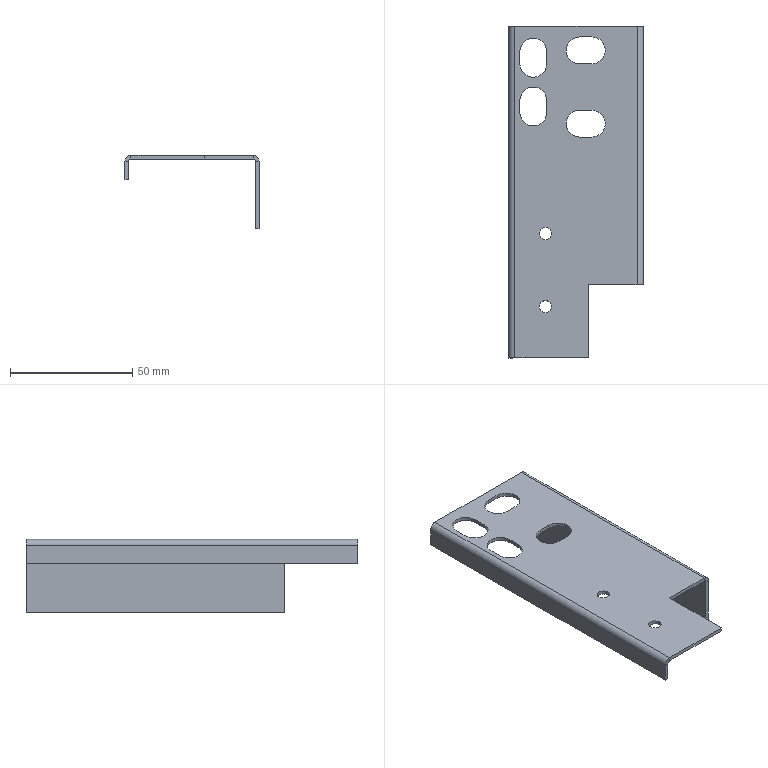Part | SolidWorks | features Cut 4, EdgeFlange 2, FlatPattern 1, SMBaseFlange 1, SheetMetal 1 | 1 solid | 46 faces | box 55 x 136 x 30 mm | volume 15241 mm3 | plane 28 | cylinder 18 | commonest cylinder face diameters 11 x10 5 x6 2 x2
STEP:
#1=CARTESIAN_POINT('',(12.,58.,-1.5));
#2=VERTEX_POINT('',#1);
#3=CARTESIAN_POINT('',(6.5,63.5,-1.5));
#4=VERTEX_POINT('',#3);
#5=CARTESIAN_POINT('',(6.5,58.,-1.5));
#6=DIRECTION('',(0.,0.,1.));
#7=DIRECTION('',(1.,0.,0.));
#8=AXIS2_PLACEMENT_3D('',#5,#6,#7);
#9=CIRCLE('',#8,5.5);
#10=EDGE_CURVE('',#2,#4,#9,.T.);
#11=ORIENTED_EDGE('',*,*,#10,.F.);
#12=CARTESIAN_POINT('',(12.,58.,0.));
#13=VERTEX_POINT('',#12);
#14=CARTESIAN_POINT('',(12.,58.,-10.));
#15=DIRECTION('',(0.,0.,1.));
#16=VECTOR('',#15,1000.);
#17=LINE('',#14,#16);
#18=EDGE_CURVE('',#2,#13,#17,.T.);
#19=ORIENTED_EDGE('',*,*,#18,.T.);
#20=CARTESIAN_POINT('',(6.5,63.5,0.));
#21=VERTEX_POINT('',#20);
#22=CARTESIAN_POINT('',(6.5,58.,0.));
#23=DIRECTION('',(0.,0.,1.));
#24=DIRECTION('',(1.,0.,0.));
#25=AXIS2_PLACEMENT_3D('',#22,#23,#24);
#26=CIRCLE('',#25,5.5);
#27=EDGE_CURVE('',#13,#21,#26,.T.);
#28=ORIENTED_EDGE('',*,*,#27,.T.);
#29=CARTESIAN_POINT('',(6.5,63.5,-10.));
#30=DIRECTION('',(0.,0.,1.));
#31=VECTOR('',#30,1000.);
#32=LINE('',#29,#31);
#33=EDGE_CURVE('',#4,#21,#32,.T.);
#34=ORIENTED_EDGE('',*,*,#33,.F.);
#35=EDGE_LOOP('',(#11,#19,#28,#34));
#36=FACE_OUTER_BOUND('',#35,.T.);
#37=CARTESIAN_POINT('',(6.5,58.,-10.));
#38=DIRECTION('',(0.,0.,1.));
#39=DIRECTION('',(1.,0.,0.));
#40=AXIS2_PLACEMENT_3D('',#37,#38,#39);
#41=CYLINDRICAL_SURFACE('',#40,5.5);
#42=ADVANCED_FACE('',(#36),#41,.F.);
#43=CARTESIAN_POINT('',(12.,28.,-1.5));
#44=VERTEX_POINT('',#43);
#45=CARTESIAN_POINT('',(6.5,33.5,-1.5));
#46=VERTEX_POINT('',#45);
#47=CARTESIAN_POINT('',(6.5,28.,-1.5));
#48=DIRECTION('',(0.,0.,1.));
#49=DIRECTION('',(1.,0.,0.));
#50=AXIS2_PLACEMENT_3D('',#47,#48,#49);
#51=CIRCLE('',#50,5.5);
#52=EDGE_CURVE('',#44,#46,#51,.T.);
#53=ORIENTED_EDGE('',*,*,#52,.F.);
#54=CARTESIAN_POINT('',(12.,28.,0.));
#55=VERTEX_POINT('',#54);
#56=CARTESIAN_POINT('',(12.,28.,-10.));
#57=DIRECTION('',(0.,0.,1.));
#58=VECTOR('',#57,1000.);
#59=LINE('',#56,#58);
#60=EDGE_CURVE('',#44,#55,#59,.T.);
#61=ORIENTED_EDGE('',*,*,#60,.T.);
#62=CARTESIAN_POINT('',(6.5,33.5,0.));
#63=VERTEX_POINT('',#62);
#64=CARTESIAN_POINT('',(6.5,28.,0.));
#65=DIRECTION('',(0.,0.,1.));
#66=DIRECTION('',(1.,0.,0.));
#67=AXIS2_PLACEMENT_3D('',#64,#65,#66);
#68=CIRCLE('',#67,5.5);
#69=EDGE_CURVE('',#55,#63,#68,.T.);
#70=ORIENTED_EDGE('',*,*,#69,.T.);
#71=CARTESIAN_POINT('',(6.5,33.5,-10.));
#72=DIRECTION('',(0.,0.,1.));
#73=VECTOR('',#72,1000.);
#74=LINE('',#71,#73);
#75=EDGE_CURVE('',#46,#63,#74,.T.);
#76=ORIENTED_EDGE('',*,*,#75,.F.);
#77=EDGE_LOOP('',(#53,#61,#70,#76));
#78=FACE_OUTER_BOUND('',#77,.T.);
#79=CARTESIAN_POINT('',(6.5,28.,-10.));
#80=DIRECTION('',(0.,0.,1.));
#81=DIRECTION('',(1.,0.,0.));
#82=AXIS2_PLACEMENT_3D('',#79,#80,#81);
#83=CYLINDRICAL_SURFACE('',#82,5.5);
#84=ADVANCED_FACE('',(#78),#83,.F.);
#85=CARTESIAN_POINT('',(-15.,-47.,-1.5));
#86=VERTEX_POINT('',#85);
#87=CARTESIAN_POINT('',(-10.,-47.,-1.5));
#88=VERTEX_POINT('',#87);
#89=CARTESIAN_POINT('',(-12.5,-47.,-1.5));
#90=DIRECTION('',(0.,0.,1.));
#91=DIRECTION('',(1.,0.,0.));
#92=AXIS2_PLACEMENT_3D('',#89,#90,#91);
#93=CIRCLE('',#92,2.5);
#94=EDGE_CURVE('',#86,#88,#93,.T.);
#95=ORIENTED_EDGE('',*,*,#94,.F.);
#96=CARTESIAN_POINT('',(-15.,-47.,0.));
#97=VERTEX_POINT('',#96);
#98=CARTESIAN_POINT('',(-15.,-47.,-10.));
#99=DIRECTION('',(0.,0.,1.));
#100=VECTOR('',#99,1000.);
#101=LINE('',#98,#100);
#102=EDGE_CURVE('',#86,#97,#101,.T.);
#103=ORIENTED_EDGE('',*,*,#102,.T.);
#104=CARTESIAN_POINT('',(-10.,-47.,0.));
#105=VERTEX_POINT('',#104);
#106=CARTESIAN_POINT('',(-12.5,-47.,0.));
#107=DIRECTION('',(0.,0.,1.));
#108=DIRECTION('',(1.,0.,0.));
#109=AXIS2_PLACEMENT_3D('',#106,#107,#108);
#110=CIRCLE('',#109,2.5);
#111=EDGE_CURVE('',#97,#105,#110,.T.);
#112=ORIENTED_EDGE('',*,*,#111,.T.);
#113=CARTESIAN_POINT('',(-10.,-47.,-10.));
#114=DIRECTION('',(0.,0.,1.));
#115=VECTOR('',#114,1000.);
#116=LINE('',#113,#115);
#117=EDGE_CURVE('',#88,#105,#116,.T.);
#118=ORIENTED_EDGE('',*,*,#117,.F.);
#119=EDGE_LOOP('',(#95,#103,#112,#118));
#120=FACE_OUTER_BOUND('',#119,.T.);
#121=CARTESIAN_POINT('',(-12.5,-47.,-10.));
#122=DIRECTION('',(0.,0.,1.));
#123=DIRECTION('',(1.,0.,0.));
#124=AXIS2_PLACEMENT_3D('',#121,#122,#123);
#125=CYLINDRICAL_SURFACE('',#124,2.5);
#126=ADVANCED_FACE('',(#120),#125,.F.);
#127=CARTESIAN_POINT('',(-15.,-17.,-1.5));
#128=VERTEX_POINT('',#127);
#129=CARTESIAN_POINT('',(-10.,-17.,-1.5));
#130=VERTEX_POINT('',#129);
#131=CARTESIAN_POINT('',(-12.5,-17.,-1.5));
#132=DIRECTION('',(0.,0.,1.));
#133=DIRECTION('',(1.,0.,0.));
#134=AXIS2_PLACEMENT_3D('',#131,#132,#133);
#135=CIRCLE('',#134,2.5);
#136=EDGE_CURVE('',#128,#130,#135,.T.);
#137=ORIENTED_EDGE('',*,*,#136,.F.);
#138=CARTESIAN_POINT('',(-15.,-17.,0.));
#139=VERTEX_POINT('',#138);
#140=CARTESIAN_POINT('',(-15.,-17.,-10.));
#141=DIRECTION('',(0.,0.,1.));
#142=VECTOR('',#141,1000.);
#143=LINE('',#140,#142);
#144=EDGE_CURVE('',#128,#139,#143,.T.);
#145=ORIENTED_EDGE('',*,*,#144,.T.);
#146=CARTESIAN_POINT('',(-10.,-17.,0.));
#147=VERTEX_POINT('',#146);
#148=CARTESIAN_POINT('',(-12.5,-17.,0.));
#149=DIRECTION('',(0.,0.,1.));
#150=DIRECTION('',(1.,0.,0.));
#151=AXIS2_PLACEMENT_3D('',#148,#149,#150);
#152=CIRCLE('',#151,2.5);
#153=EDGE_CURVE('',#139,#147,#152,.T.);
#154=ORIENTED_EDGE('',*,*,#153,.T.);
#155=CARTESIAN_POINT('',(-10.,-17.,-10.));
#156=DIRECTION('',(0.,0.,1.));
#157=VECTOR('',#156,1000.);
#158=LINE('',#155,#157);
#159=EDGE_CURVE('',#130,#147,#158,.T.);
#160=ORIENTED_EDGE('',*,*,#159,.F.);
#161=EDGE_LOOP('',(#137,#145,#154,#160));
#162=FACE_OUTER_BOUND('',#161,.T.);
#163=CARTESIAN_POINT('',(-12.5,-17.,-10.));
#164=DIRECTION('',(0.,0.,1.));
#165=DIRECTION('',(1.,0.,0.));
#166=AXIS2_PLACEMENT_3D('',#163,#164,#165);
#167=CYLINDRICAL_SURFACE('',#166,2.5);
#168=ADVANCED_FACE('',(#162),#167,.F.);
#169=CARTESIAN_POINT('',(27.5,-38.,-30.));
#170=VERTEX_POINT('',#169);
#171=CARTESIAN_POINT('',(27.5,-38.,-2.5));
#172=VERTEX_POINT('',#171);
#173=CARTESIAN_POINT('',(27.5,-38.,-30.));
#174=DIRECTION('',(0.,0.,1.));
#175=VECTOR('',#174,1000.);
#176=LINE('',#173,#175);
#177=EDGE_CURVE('',#170,#172,#176,.T.);
#178=ORIENTED_EDGE('',*,*,#177,.T.);
#179=CARTESIAN_POINT('',(26.,-38.,-2.5));
#180=VERTEX_POINT('',#179);
#181=CARTESIAN_POINT('',(27.5,-38.,-2.5));
#182=DIRECTION('',(-1.,0.,0.));
#183=VECTOR('',#182,1000.);
#184=LINE('',#181,#183);
#185=EDGE_CURVE('',#172,#180,#184,.T.);
#186=ORIENTED_EDGE('',*,*,#185,.T.);
#187=CARTESIAN_POINT('',(26.,-38.,-30.));
#188=VERTEX_POINT('',#187);
#189=CARTESIAN_POINT('',(26.,-38.,0.));
#190=DIRECTION('',(0.,0.,1.));
#191=VECTOR('',#190,1000.);
#192=LINE('',#189,#191);
#193=EDGE_CURVE('',#188,#180,#192,.T.);
#194=ORIENTED_EDGE('',*,*,#193,.F.);
#195=CARTESIAN_POINT('',(27.5,-38.,-30.));
#196=DIRECTION('',(-1.,0.,0.));
#197=VECTOR('',#196,1000.);
#198=LINE('',#195,#197);
#199=EDGE_CURVE('',#170,#188,#198,.T.);
#200=ORIENTED_EDGE('',*,*,#199,.F.);
#201=EDGE_LOOP('',(#178,#186,#194,#200));
#202=FACE_OUTER_BOUND('',#201,.T.);
#203=CARTESIAN_POINT('',(27.5,-38.,-30.));
#204=DIRECTION('',(0.,1.,0.));
#205=DIRECTION('',(-1.,0.,0.));
#206=AXIS2_PLACEMENT_3D('',#203,#204,#205);
#207=PLANE('',#206);
#208=ADVANCED_FACE('',(#202),#207,.F.);
#209=CARTESIAN_POINT('',(25.,-38.,-1.5));
#210=VERTEX_POINT('',#209);
#211=CARTESIAN_POINT('',(5.,-38.,-1.5));
#212=VERTEX_POINT('',#211);
#213=CARTESIAN_POINT('',(0.,-38.,-1.5));
#214=DIRECTION('',(-1.,0.,0.));
#215=VECTOR('',#214,1000.);
#216=LINE('',#213,#215);
#217=EDGE_CURVE('',#210,#212,#216,.T.);
#218=ORIENTED_EDGE('',*,*,#217,.F.);
#219=CARTESIAN_POINT('',(25.,-38.,0.));
#220=VERTEX_POINT('',#219);
#221=CARTESIAN_POINT('',(25.,-38.,-1.5));
#222=DIRECTION('',(0.,0.,1.));
#223=VECTOR('',#222,1000.);
#224=LINE('',#221,#223);
#225=EDGE_CURVE('',#210,#220,#224,.T.);
#226=ORIENTED_EDGE('',*,*,#225,.T.);
#227=CARTESIAN_POINT('',(5.,-38.,0.));
#228=VERTEX_POINT('',#227);
#229=CARTESIAN_POINT('',(0.,-38.,0.));
#230=DIRECTION('',(-1.,0.,0.));
#231=VECTOR('',#230,1000.);
#232=LINE('',#229,#231);
#233=EDGE_CURVE('',#220,#228,#232,.T.);
#234=ORIENTED_EDGE('',*,*,#233,.T.);
#235=CARTESIAN_POINT('',(5.,-38.,-30.));
#236=DIRECTION('',(0.,0.,1.));
#237=VECTOR('',#236,1000.);
#238=LINE('',#235,#237);
#239=EDGE_CURVE('',#212,#228,#238,.T.);
#240=ORIENTED_EDGE('',*,*,#239,.F.);
#241=EDGE_LOOP('',(#218,#226,#234,#240));
#242=FACE_OUTER_BOUND('',#241,.T.);
#243=CARTESIAN_POINT('',(27.5,-38.,-30.));
#244=DIRECTION('',(0.,1.,0.));
#245=DIRECTION('',(-1.,0.,0.));
#246=AXIS2_PLACEMENT_3D('',#243,#244,#245);
#247=PLANE('',#246);
#248=ADVANCED_FACE('',(#242),#247,.F.);
#249=CARTESIAN_POINT('',(-12.,52.5,-1.5));
#250=VERTEX_POINT('',#249);
#251=CARTESIAN_POINT('',(-12.,57.5,-1.5));
#252=VERTEX_POINT('',#251);
#253=CARTESIAN_POINT('',(-12.,0.,-1.5));
#254=DIRECTION('',(0.,1.,0.));
#255=VECTOR('',#254,1000.);
#256=LINE('',#253,#255);
#257=EDGE_CURVE('',#250,#252,#256,.T.);
#258=ORIENTED_EDGE('',*,*,#257,.T.);
#259=CARTESIAN_POINT('',(-23.,57.5,-1.5));
#260=VERTEX_POINT('',#259);
#261=CARTESIAN_POINT('',(-17.5,57.5,-1.5));
#262=DIRECTION('',(0.,0.,1.));
#263=DIRECTION('',(1.,0.,0.));
#264=AXIS2_PLACEMENT_3D('',#261,#262,#263);
#265=CIRCLE('',#264,5.5);
#266=EDGE_CURVE('',#252,#260,#265,.T.);
#267=ORIENTED_EDGE('',*,*,#266,.T.);
#268=CARTESIAN_POINT('',(-23.,52.5,-1.5));
#269=VERTEX_POINT('',#268);
#270=CARTESIAN_POINT('',(-23.,0.,-1.5));
#271=DIRECTION('',(0.,-1.,0.));
#272=VECTOR('',#271,1000.);
#273=LINE('',#270,#272);
#274=EDGE_CURVE('',#260,#269,#273,.T.);
#275=ORIENTED_EDGE('',*,*,#274,.T.);
#276=CARTESIAN_POINT('',(-17.5,52.5,-1.5));
#277=DIRECTION('',(0.,0.,1.));
#278=DIRECTION('',(1.,0.,0.));
#279=AXIS2_PLACEMENT_3D('',#276,#277,#278);
#280=CIRCLE('',#279,5.5);
#281=EDGE_CURVE('',#269,#250,#280,.T.);
#282=ORIENTED_EDGE('',*,*,#281,.T.);
#283=EDGE_LOOP('',(#258,#267,#275,#282));
#284=FACE_BOUND('',#283,.T.);
#285=CARTESIAN_POINT('',(-12.,32.5,-1.5));
#286=VERTEX_POINT('',#285);
#287=CARTESIAN_POINT('',(-12.,37.5,-1.5));
#288=VERTEX_POINT('',#287);
#289=CARTESIAN_POINT('',(-12.,0.,-1.5));
#290=DIRECTION('',(0.,1.,0.));
#291=VECTOR('',#290,1000.);
#292=LINE('',#289,#291);
#293=EDGE_CURVE('',#286,#288,#292,.T.);
#294=ORIENTED_EDGE('',*,*,#293,.T.);
#295=CARTESIAN_POINT('',(-23.,37.5,-1.5));
#296=VERTEX_POINT('',#295);
#297=CARTESIAN_POINT('',(-17.5,37.5,-1.5));
#298=DIRECTION('',(0.,0.,1.));
#299=DIRECTION('',(1.,0.,0.));
#300=AXIS2_PLACEMENT_3D('',#297,#298,#299);
#301=CIRCLE('',#300,5.5);
#302=EDGE_CURVE('',#288,#296,#301,.T.);
#303=ORIENTED_EDGE('',*,*,#302,.T.);
#304=CARTESIAN_POINT('',(-23.,32.5,-1.5));
#305=VERTEX_POINT('',#304);
#306=CARTESIAN_POINT('',(-23.,0.,-1.5));
#307=DIRECTION('',(0.,-1.,0.));
#308=VECTOR('',#307,1000.);
#309=LINE('',#306,#308);
#310=EDGE_CURVE('',#296,#305,#309,.T.);
#311=ORIENTED_EDGE('',*,*,#310,.T.);
#312=CARTESIAN_POINT('',(-17.5,32.5,-1.5));
#313=DIRECTION('',(0.,0.,1.));
#314=DIRECTION('',(1.,0.,0.));
#315=AXIS2_PLACEMENT_3D('',#312,#313,#314);
#316=CIRCLE('',#315,5.5);
#317=EDGE_CURVE('',#305,#286,#316,.T.);
#318=ORIENTED_EDGE('',*,*,#317,.T.);
#319=EDGE_LOOP('',(#294,#303,#311,#318));
#320=FACE_BOUND('',#319,.T.);
#321=CARTESIAN_POINT('',(1.5,63.5,-1.5));
#322=VERTEX_POINT('',#321);
#323=CARTESIAN_POINT('',(0.,63.5,-1.5));
#324=DIRECTION('',(-1.,0.,0.));
#325=VECTOR('',#324,1000.);
#326=LINE('',#323,#325);
#327=EDGE_CURVE('',#4,#322,#326,.T.);
#328=ORIENTED_EDGE('',*,*,#327,.T.);
#329=CARTESIAN_POINT('',(1.5,52.5,-1.5));
#330=VERTEX_POINT('',#329);
#331=CARTESIAN_POINT('',(1.5,58.,-1.5));
#332=DIRECTION('',(0.,0.,1.));
#333=DIRECTION('',(1.,0.,0.));
#334=AXIS2_PLACEMENT_3D('',#331,#332,#333);
#335=CIRCLE('',#334,5.5);
#336=EDGE_CURVE('',#322,#330,#335,.T.);
#337=ORIENTED_EDGE('',*,*,#336,.T.);
#338=CARTESIAN_POINT('',(6.5,52.5,-1.5));
#339=VERTEX_POINT('',#338);
#340=CARTESIAN_POINT('',(0.,52.5,-1.5));
#341=DIRECTION('',(1.,0.,0.));
#342=VECTOR('',#341,1000.);
#343=LINE('',#340,#342);
#344=EDGE_CURVE('',#330,#339,#343,.T.);
#345=ORIENTED_EDGE('',*,*,#344,.T.);
#346=CARTESIAN_POINT('',(6.5,58.,-1.5));
#347=DIRECTION('',(0.,0.,1.));
#348=DIRECTION('',(1.,0.,0.));
#349=AXIS2_PLACEMENT_3D('',#346,#347,#348);
#350=CIRCLE('',#349,5.5);
#351=EDGE_CURVE('',#339,#2,#350,.T.);
#352=ORIENTED_EDGE('',*,*,#351,.T.);
#353=ORIENTED_EDGE('',*,*,#10,.T.);
#354=EDGE_LOOP('',(#328,#337,#345,#352,#353));
#355=FACE_BOUND('',#354,.T.);
#356=CARTESIAN_POINT('',(1.5,33.5,-1.5));
#357=VERTEX_POINT('',#356);
#358=CARTESIAN_POINT('',(0.,33.5,-1.5));
#359=DIRECTION('',(-1.,0.,0.));
#360=VECTOR('',#359,1000.);
#361=LINE('',#358,#360);
#362=EDGE_CURVE('',#46,#357,#361,.T.);
#363=ORIENTED_EDGE('',*,*,#362,.T.);
#364=CARTESIAN_POINT('',(1.5,22.5,-1.5));
#365=VERTEX_POINT('',#364);
#366=CARTESIAN_POINT('',(1.5,28.,-1.5));
#367=DIRECTION('',(0.,0.,1.));
#368=DIRECTION('',(1.,0.,0.));
#369=AXIS2_PLACEMENT_3D('',#366,#367,#368);
#370=CIRCLE('',#369,5.5);
#371=EDGE_CURVE('',#357,#365,#370,.T.);
#372=ORIENTED_EDGE('',*,*,#371,.T.);
#373=CARTESIAN_POINT('',(6.5,22.5,-1.5));
#374=VERTEX_POINT('',#373);
#375=CARTESIAN_POINT('',(0.,22.5,-1.5));
#376=DIRECTION('',(1.,0.,0.));
#377=VECTOR('',#376,1000.);
#378=LINE('',#375,#377);
#379=EDGE_CURVE('',#365,#374,#378,.T.);
#380=ORIENTED_EDGE('',*,*,#379,.T.);
#381=CARTESIAN_POINT('',(6.5,28.,-1.5));
#382=DIRECTION('',(0.,0.,1.));
#383=DIRECTION('',(1.,0.,0.));
#384=AXIS2_PLACEMENT_3D('',#381,#382,#383);
#385=CIRCLE('',#384,5.5);
#386=EDGE_CURVE('',#374,#44,#385,.T.);
#387=ORIENTED_EDGE('',*,*,#386,.T.);
#388=ORIENTED_EDGE('',*,*,#52,.T.);
#389=EDGE_LOOP('',(#363,#372,#380,#387,#388));
#390=FACE_BOUND('',#389,.T.);
#391=CARTESIAN_POINT('',(-12.5,-47.,-1.5));
#392=DIRECTION('',(0.,0.,1.));
#393=DIRECTION('',(1.,0.,0.));
#394=AXIS2_PLACEMENT_3D('',#391,#392,#393);
#395=CIRCLE('',#394,2.5);
#396=EDGE_CURVE('',#88,#86,#395,.T.);
#397=ORIENTED_EDGE('',*,*,#396,.T.);
#398=ORIENTED_EDGE('',*,*,#94,.T.);
#399=EDGE_LOOP('',(#397,#398));
#400=FACE_BOUND('',#399,.T.);
#401=CARTESIAN_POINT('',(-12.5,-17.,-1.5));
#402=DIRECTION('',(0.,0.,1.));
#403=DIRECTION('',(1.,0.,0.));
#404=AXIS2_PLACEMENT_3D('',#401,#402,#403);
#405=CIRCLE('',#404,2.5);
#406=EDGE_CURVE('',#130,#128,#405,.T.);
#407=ORIENTED_EDGE('',*,*,#406,.T.);
#408=ORIENTED_EDGE('',*,*,#136,.T.);
#409=EDGE_LOOP('',(#407,#408));
#410=FACE_BOUND('',#409,.T.);
#411=ORIENTED_EDGE('',*,*,#217,.T.);
#412=CARTESIAN_POINT('',(5.,-68.,-1.5));
#413=VERTEX_POINT('',#412);
#414=CARTESIAN_POINT('',(5.,0.,-1.5));
#415=DIRECTION('',(0.,-1.,0.));
#416=VECTOR('',#415,1000.);
#417=LINE('',#414,#416);
#418=EDGE_CURVE('',#212,#413,#417,.T.);
#419=ORIENTED_EDGE('',*,*,#418,.T.);
#420=CARTESIAN_POINT('',(-25.,-68.,-1.5));
#421=VERTEX_POINT('',#420);
#422=CARTESIAN_POINT('',(-27.5,-68.,-1.5));
#423=DIRECTION('',(1.,0.,0.));
#424=VECTOR('',#423,1000.);
#425=LINE('',#422,#424);
#426=EDGE_CURVE('',#421,#413,#425,.T.);
#427=ORIENTED_EDGE('',*,*,#426,.F.);
#428=CARTESIAN_POINT('',(-25.,68.,-1.5));
#429=VERTEX_POINT('',#428);
#430=CARTESIAN_POINT('',(-25.,68.,-1.5));
#431=DIRECTION('',(0.,-1.,0.));
#432=VECTOR('',#431,1000.);
#433=LINE('',#430,#432);
#434=EDGE_CURVE('',#429,#421,#433,.T.);
#435=ORIENTED_EDGE('',*,*,#434,.F.);
#436=CARTESIAN_POINT('',(25.,68.,-1.5));
#437=VERTEX_POINT('',#436);
#438=CARTESIAN_POINT('',(-27.5,68.,-1.5));
#439=DIRECTION('',(-1.,0.,0.));
#440=VECTOR('',#439,1000.);
#441=LINE('',#438,#440);
#442=EDGE_CURVE('',#437,#429,#441,.T.);
#443=ORIENTED_EDGE('',*,*,#442,.F.);
#444=CARTESIAN_POINT('',(25.,-68.,-1.5));
#445=DIRECTION('',(0.,1.,0.));
#446=VECTOR('',#445,1000.);
#447=LINE('',#444,#446);
#448=EDGE_CURVE('',#210,#437,#447,.T.);
#449=ORIENTED_EDGE('',*,*,#448,.F.);
#450=EDGE_LOOP('',(#411,#419,#427,#435,#443,#449));
#451=FACE_OUTER_BOUND('',#450,.T.);
#452=CARTESIAN_POINT('',(0.,0.,-1.5));
#453=DIRECTION('',(0.,0.,1.));
#454=DIRECTION('',(1.,0.,0.));
#455=AXIS2_PLACEMENT_3D('',#452,#453,#454);
#456=PLANE('',#455);
#457=ADVANCED_FACE('',(#284,#320,#355,#390,#400,#410,#451),#456,.F.);
#458=CARTESIAN_POINT('',(-12.,57.5,0.));
#459=VERTEX_POINT('',#458);
#460=CARTESIAN_POINT('',(-23.,57.5,0.));
#461=VERTEX_POINT('',#460);
#462=CARTESIAN_POINT('',(-17.5,57.5,0.));
#463=DIRECTION('',(0.,0.,1.));
#464=DIRECTION('',(1.,0.,0.));
#465=AXIS2_PLACEMENT_3D('',#462,#463,#464);
#466=CIRCLE('',#465,5.5);
#467=EDGE_CURVE('',#459,#461,#466,.T.);
#468=ORIENTED_EDGE('',*,*,#467,.F.);
#469=CARTESIAN_POINT('',(-12.,52.5,0.));
#470=VERTEX_POINT('',#469);
#471=CARTESIAN_POINT('',(-12.,57.5,0.));
#472=DIRECTION('',(0.,1.,0.));
#473=VECTOR('',#472,1000.);
#474=LINE('',#471,#473);
#475=EDGE_CURVE('',#470,#459,#474,.T.);
#476=ORIENTED_EDGE('',*,*,#475,.F.);
#477=CARTESIAN_POINT('',(-23.,52.5,0.));
#478=VERTEX_POINT('',#477);
#479=CARTESIAN_POINT('',(-17.5,52.5,0.));
#480=DIRECTION('',(0.,0.,1.));
#481=DIRECTION('',(1.,0.,0.));
#482=AXIS2_PLACEMENT_3D('',#479,#480,#481);
#483=CIRCLE('',#482,5.5);
#484=EDGE_CURVE('',#478,#470,#483,.T.);
#485=ORIENTED_EDGE('',*,*,#484,.F.);
#486=CARTESIAN_POINT('',(-23.,57.5,0.));
#487=DIRECTION('',(0.,-1.,0.));
#488=VECTOR('',#487,1000.);
#489=LINE('',#486,#488);
#490=EDGE_CURVE('',#461,#478,#489,.T.);
#491=ORIENTED_EDGE('',*,*,#490,.F.);
#492=EDGE_LOOP('',(#468,#476,#485,#491));
#493=FACE_BOUND('',#492,.T.);
#494=CARTESIAN_POINT('',(-12.,37.5,0.));
#495=VERTEX_POINT('',#494);
#496=CARTESIAN_POINT('',(-23.,37.5,0.));
#497=VERTEX_POINT('',#496);
#498=CARTESIAN_POINT('',(-17.5,37.5,0.));
#499=DIRECTION('',(0.,0.,1.));
#500=DIRECTION('',(1.,0.,0.));
#501=AXIS2_PLACEMENT_3D('',#498,#499,#500);
#502=CIRCLE('',#501,5.5);
#503=EDGE_CURVE('',#495,#497,#502,.T.);
#504=ORIENTED_EDGE('',*,*,#503,.F.);
#505=CARTESIAN_POINT('',(-12.,32.5,0.));
#506=VERTEX_POINT('',#505);
#507=CARTESIAN_POINT('',(-12.,37.5,0.));
#508=DIRECTION('',(0.,1.,0.));
#509=VECTOR('',#508,1000.);
#510=LINE('',#507,#509);
#511=EDGE_CURVE('',#506,#495,#510,.T.);
#512=ORIENTED_EDGE('',*,*,#511,.F.);
#513=CARTESIAN_POINT('',(-23.,32.5,0.));
#514=VERTEX_POINT('',#513);
#515=CARTESIAN_POINT('',(-17.5,32.5,0.));
#516=DIRECTION('',(0.,0.,1.));
#517=DIRECTION('',(1.,0.,0.));
#518=AXIS2_PLACEMENT_3D('',#515,#516,#517);
#519=CIRCLE('',#518,5.5);
#520=EDGE_CURVE('',#514,#506,#519,.T.);
#521=ORIENTED_EDGE('',*,*,#520,.F.);
#522=CARTESIAN_POINT('',(-23.,37.5,0.));
#523=DIRECTION('',(0.,-1.,0.));
#524=VECTOR('',#523,1000.);
#525=LINE('',#522,#524);
#526=EDGE_CURVE('',#497,#514,#525,.T.);
#527=ORIENTED_EDGE('',*,*,#526,.F.);
#528=EDGE_LOOP('',(#504,#512,#521,#527));
#529=FACE_BOUND('',#528,.T.);
#530=CARTESIAN_POINT('',(1.5,63.5,0.));
#531=VERTEX_POINT('',#530);
#532=CARTESIAN_POINT('',(1.5,52.5,0.));
#533=VERTEX_POINT('',#532);
#534=CARTESIAN_POINT('',(1.5,58.,0.));
#535=DIRECTION('',(0.,0.,1.));
#536=DIRECTION('',(1.,0.,0.));
#537=AXIS2_PLACEMENT_3D('',#534,#535,#536);
#538=CIRCLE('',#537,5.5);
#539=EDGE_CURVE('',#531,#533,#538,.T.);
#540=ORIENTED_EDGE('',*,*,#539,.F.);
#541=CARTESIAN_POINT('',(1.5,63.5,0.));
#542=DIRECTION('',(-1.,0.,0.));
#543=VECTOR('',#542,1000.);
#544=LINE('',#541,#543);
#545=EDGE_CURVE('',#21,#531,#544,.T.);
#546=ORIENTED_EDGE('',*,*,#545,.F.);
#547=ORIENTED_EDGE('',*,*,#27,.F.);
#548=CARTESIAN_POINT('',(6.5,52.5,0.));
#549=VERTEX_POINT('',#548);
#550=CARTESIAN_POINT('',(6.5,58.,0.));
#551=DIRECTION('',(0.,0.,1.));
#552=DIRECTION('',(1.,0.,0.));
#553=AXIS2_PLACEMENT_3D('',#550,#551,#552);
#554=CIRCLE('',#553,5.5);
#555=EDGE_CURVE('',#549,#13,#554,.T.);
#556=ORIENTED_EDGE('',*,*,#555,.F.);
#557=CARTESIAN_POINT('',(1.5,52.5,0.));
#558=DIRECTION('',(1.,0.,0.));
#559=VECTOR('',#558,1000.);
#560=LINE('',#557,#559);
#561=EDGE_CURVE('',#533,#549,#560,.T.);
#562=ORIENTED_EDGE('',*,*,#561,.F.);
#563=EDGE_LOOP('',(#540,#546,#547,#556,#562));
#564=FACE_BOUND('',#563,.T.);
#565=CARTESIAN_POINT('',(1.5,33.5,0.));
#566=VERTEX_POINT('',#565);
#567=CARTESIAN_POINT('',(1.5,22.5,0.));
#568=VERTEX_POINT('',#567);
#569=CARTESIAN_POINT('',(1.5,28.,0.));
#570=DIRECTION('',(0.,0.,1.));
#571=DIRECTION('',(1.,0.,0.));
#572=AXIS2_PLACEMENT_3D('',#569,#570,#571);
#573=CIRCLE('',#572,5.5);
#574=EDGE_CURVE('',#566,#568,#573,.T.);
#575=ORIENTED_EDGE('',*,*,#574,.F.);
#576=CARTESIAN_POINT('',(1.5,33.5,0.));
#577=DIRECTION('',(-1.,0.,0.));
#578=VECTOR('',#577,1000.);
#579=LINE('',#576,#578);
#580=EDGE_CURVE('',#63,#566,#579,.T.);
#581=ORIENTED_EDGE('',*,*,#580,.F.);
#582=ORIENTED_EDGE('',*,*,#69,.F.);
#583=CARTESIAN_POINT('',(6.5,22.5,0.));
#584=VERTEX_POINT('',#583);
#585=CARTESIAN_POINT('',(6.5,28.,0.));
#586=DIRECTION('',(0.,0.,1.));
#587=DIRECTION('',(1.,0.,0.));
#588=AXIS2_PLACEMENT_3D('',#585,#586,#587);
#589=CIRCLE('',#588,5.5);
#590=EDGE_CURVE('',#584,#55,#589,.T.);
#591=ORIENTED_EDGE('',*,*,#590,.F.);
#592=CARTESIAN_POINT('',(1.5,22.5,0.));
#593=DIRECTION('',(1.,0.,0.));
#594=VECTOR('',#593,1000.);
#595=LINE('',#592,#594);
#596=EDGE_CURVE('',#568,#584,#595,.T.);
#597=ORIENTED_EDGE('',*,*,#596,.F.);
#598=EDGE_LOOP('',(#575,#581,#582,#591,#597));
#599=FACE_BOUND('',#598,.T.);
#600=CARTESIAN_POINT('',(-12.5,-47.,0.));
#601=DIRECTION('',(0.,0.,1.));
#602=DIRECTION('',(1.,0.,0.));
#603=AXIS2_PLACEMENT_3D('',#600,#601,#602);
#604=CIRCLE('',#603,2.5);
#605=EDGE_CURVE('',#105,#97,#604,.T.);
#606=ORIENTED_EDGE('',*,*,#605,.F.);
#607=ORIENTED_EDGE('',*,*,#111,.F.);
#608=EDGE_LOOP('',(#606,#607));
#609=FACE_BOUND('',#608,.T.);
#610=CARTESIAN_POINT('',(-12.5,-17.,0.));
#611=DIRECTION('',(0.,0.,1.));
#612=DIRECTION('',(1.,0.,0.));
#613=AXIS2_PLACEMENT_3D('',#610,#611,#612);
#614=CIRCLE('',#613,2.5);
#615=EDGE_CURVE('',#147,#139,#614,.T.);
#616=ORIENTED_EDGE('',*,*,#615,.F.);
#617=ORIENTED_EDGE('',*,*,#153,.F.);
#618=EDGE_LOOP('',(#616,#617));
#619=FACE_BOUND('',#618,.T.);
#620=CARTESIAN_POINT('',(5.,-68.,0.));
#621=VERTEX_POINT('',#620);
#622=CARTESIAN_POINT('',(5.,0.,0.));
#623=DIRECTION('',(0.,-1.,0.));
#624=VECTOR('',#623,1000.);
#625=LINE('',#622,#624);
#626=EDGE_CURVE('',#228,#621,#625,.T.);
#627=ORIENTED_EDGE('',*,*,#626,.F.);
#628=ORIENTED_EDGE('',*,*,#233,.F.);
#629=CARTESIAN_POINT('',(25.,68.,0.));
#630=VERTEX_POINT('',#629);
#631=CARTESIAN_POINT('',(25.,-68.,0.));
#632=DIRECTION('',(0.,1.,0.));
#633=VECTOR('',#632,1000.);
#634=LINE('',#631,#633);
#635=EDGE_CURVE('',#220,#630,#634,.T.);
#636=ORIENTED_EDGE('',*,*,#635,.T.);
#637=CARTESIAN_POINT('',(-25.,68.,0.));
#638=VERTEX_POINT('',#637);
#639=CARTESIAN_POINT('',(-27.5,68.,0.));
#640=DIRECTION('',(-1.,0.,0.));
#641=VECTOR('',#640,1000.);
#642=LINE('',#639,#641);
#643=EDGE_CURVE('',#630,#638,#642,.T.);
#644=ORIENTED_EDGE('',*,*,#643,.T.);
#645=CARTESIAN_POINT('',(-25.,-68.,0.));
#646=VERTEX_POINT('',#645);
#647=CARTESIAN_POINT('',(-25.,68.,0.));
#648=DIRECTION('',(0.,-1.,0.));
#649=VECTOR('',#648,1000.);
#650=LINE('',#647,#649);
#651=EDGE_CURVE('',#638,#646,#650,.T.);
#652=ORIENTED_EDGE('',*,*,#651,.T.);
#653=CARTESIAN_POINT('',(-27.5,-68.,0.));
#654=DIRECTION('',(1.,0.,0.));
#655=VECTOR('',#654,1000.);
#656=LINE('',#653,#655);
#657=EDGE_CURVE('',#646,#621,#656,.T.);
#658=ORIENTED_EDGE('',*,*,#657,.T.);
#659=EDGE_LOOP('',(#627,#628,#636,#644,#652,#658));
#660=FACE_OUTER_BOUND('',#659,.T.);
#661=CARTESIAN_POINT('',(0.,0.,0.));
#662=DIRECTION('',(0.,0.,1.));
#663=DIRECTION('',(1.,0.,0.));
#664=AXIS2_PLACEMENT_3D('',#661,#662,#663);
#665=PLANE('',#664);
#666=ADVANCED_FACE('',(#493,#529,#564,#599,#609,#619,#660),#665,.T.);
#667=ORIENTED_EDGE('',*,*,#442,.T.);
#668=CARTESIAN_POINT('',(-25.,68.,-1.5));
#669=DIRECTION('',(0.,0.,1.));
#670=VECTOR('',#669,1000.);
#671=LINE('',#668,#670);
#672=EDGE_CURVE('',#429,#638,#671,.T.);
#673=ORIENTED_EDGE('',*,*,#672,.T.);
#674=ORIENTED_EDGE('',*,*,#643,.F.);
#675=CARTESIAN_POINT('',(25.,68.,-1.5));
#676=DIRECTION('',(0.,0.,1.));
#677=VECTOR('',#676,1000.);
#678=LINE('',#675,#677);
#679=EDGE_CURVE('',#437,#630,#678,.T.);
#680=ORIENTED_EDGE('',*,*,#679,.F.);
#681=EDGE_LOOP('',(#667,#673,#674,#680));
#682=FACE_OUTER_BOUND('',#681,.T.);
#683=CARTESIAN_POINT('',(-27.5,68.,-1.5));
#684=DIRECTION('',(0.,1.,0.));
#685=DIRECTION('',(0.,0.,1.));
#686=AXIS2_PLACEMENT_3D('',#683,#684,#685);
#687=PLANE('',#686);
#688=ADVANCED_FACE('',(#682),#687,.T.);
#689=CARTESIAN_POINT('',(5.,-68.,-30.));
#690=DIRECTION('',(0.,0.,1.));
#691=VECTOR('',#690,1000.);
#692=LINE('',#689,#691);
#693=EDGE_CURVE('',#413,#621,#692,.T.);
#694=ORIENTED_EDGE('',*,*,#693,.T.);
#695=ORIENTED_EDGE('',*,*,#657,.F.);
#696=CARTESIAN_POINT('',(-25.,-68.,-1.5));
#697=DIRECTION('',(0.,0.,1.));
#698=VECTOR('',#697,1000.);
#699=LINE('',#696,#698);
#700=EDGE_CURVE('',#421,#646,#699,.T.);
#701=ORIENTED_EDGE('',*,*,#700,.F.);
#702=ORIENTED_EDGE('',*,*,#426,.T.);
#703=EDGE_LOOP('',(#694,#695,#701,#702));
#704=FACE_OUTER_BOUND('',#703,.T.);
#705=CARTESIAN_POINT('',(-27.5,-68.,-1.5));
#706=DIRECTION('',(0.,-1.,0.));
#707=DIRECTION('',(0.,0.,-1.));
#708=AXIS2_PLACEMENT_3D('',#705,#706,#707);
#709=PLANE('',#708);
#710=ADVANCED_FACE('',(#704),#709,.T.);
#711=CARTESIAN_POINT('',(26.,68.,-2.5));
#712=VERTEX_POINT('',#711);
#713=CARTESIAN_POINT('',(27.5,68.,-2.5));
#714=VERTEX_POINT('',#713);
#715=CARTESIAN_POINT('',(27.5,68.,-2.5));
#716=DIRECTION('',(1.,0.,0.));
#717=VECTOR('',#716,1000.);
#718=LINE('',#715,#717);
#719=EDGE_CURVE('',#712,#714,#718,.T.);
#720=ORIENTED_EDGE('',*,*,#719,.F.);
#721=CARTESIAN_POINT('',(25.,68.,-2.5));
#722=DIRECTION('',(0.,1.,0.));
#723=DIRECTION('',(0.,0.,-1.));
#724=AXIS2_PLACEMENT_3D('',#721,#722,#723);
#725=CIRCLE('',#724,1.);
#726=EDGE_CURVE('',#437,#712,#725,.T.);
#727=ORIENTED_EDGE('',*,*,#726,.F.);
#728=ORIENTED_EDGE('',*,*,#679,.T.);
#729=CARTESIAN_POINT('',(25.,68.,-2.5));
#730=DIRECTION('',(0.,1.,0.));
#731=DIRECTION('',(0.,0.,-1.));
#732=AXIS2_PLACEMENT_3D('',#729,#730,#731);
#733=CIRCLE('',#732,2.5);
#734=EDGE_CURVE('',#630,#714,#733,.T.);
#735=ORIENTED_EDGE('',*,*,#734,.T.);
#736=EDGE_LOOP('',(#720,#727,#728,#735));
#737=FACE_OUTER_BOUND('',#736,.T.);
#738=CARTESIAN_POINT('',(25.,68.,-2.5));
#739=DIRECTION('',(0.,1.,0.));
#740=DIRECTION('',(0.,0.,1.));
#741=AXIS2_PLACEMENT_3D('',#738,#739,#740);
#742=PLANE('',#741);
#743=ADVANCED_FACE('',(#737),#742,.T.);
#744=CARTESIAN_POINT('',(25.,-38.,-2.5));
#745=DIRECTION('',(0.,-1.,0.));
#746=DIRECTION('',(-1.,0.,0.));
#747=AXIS2_PLACEMENT_3D('',#744,#745,#746);
#748=CIRCLE('',#747,2.5);
#749=EDGE_CURVE('',#172,#220,#748,.T.);
#750=ORIENTED_EDGE('',*,*,#749,.F.);
#751=CARTESIAN_POINT('',(27.5,0.,-2.5));
#752=DIRECTION('',(0.,-1.,0.));
#753=VECTOR('',#752,1000.);
#754=LINE('',#751,#753);
#755=EDGE_CURVE('',#714,#172,#754,.T.);
#756=ORIENTED_EDGE('',*,*,#755,.F.);
#757=ORIENTED_EDGE('',*,*,#734,.F.);
#758=ORIENTED_EDGE('',*,*,#635,.F.);
#759=EDGE_LOOP('',(#750,#756,#757,#758));
#760=FACE_OUTER_BOUND('',#759,.T.);
#761=CARTESIAN_POINT('',(25.,-68.,-2.5));
#762=DIRECTION('',(0.,-1.,0.));
#763=DIRECTION('',(1.,0.,0.));
#764=AXIS2_PLACEMENT_3D('',#761,#762,#763);
#765=CYLINDRICAL_SURFACE('',#764,2.5);
#766=ADVANCED_FACE('',(#760),#765,.T.);
#767=CARTESIAN_POINT('',(26.,68.,-2.5));
#768=DIRECTION('',(0.,-1.,0.));
#769=VECTOR('',#768,1000.);
#770=LINE('',#767,#769);
#771=EDGE_CURVE('',#712,#180,#770,.T.);
#772=ORIENTED_EDGE('',*,*,#771,.T.);
#773=CARTESIAN_POINT('',(25.,-38.,-2.5));
#774=DIRECTION('',(0.,-1.,0.));
#775=DIRECTION('',(-1.,0.,0.));
#776=AXIS2_PLACEMENT_3D('',#773,#774,#775);
#777=CIRCLE('',#776,1.);
#778=EDGE_CURVE('',#180,#210,#777,.T.);
#779=ORIENTED_EDGE('',*,*,#778,.T.);
#780=ORIENTED_EDGE('',*,*,#448,.T.);
#781=ORIENTED_EDGE('',*,*,#726,.T.);
#782=EDGE_LOOP('',(#772,#779,#780,#781));
#783=FACE_OUTER_BOUND('',#782,.T.);
#784=CARTESIAN_POINT('',(25.,-68.,-2.5));
#785=DIRECTION('',(0.,-1.,0.));
#786=DIRECTION('',(1.,0.,0.));
#787=AXIS2_PLACEMENT_3D('',#784,#785,#786);
#788=CYLINDRICAL_SURFACE('',#787,1.);
#789=ADVANCED_FACE('',(#783),#788,.F.);
#790=CARTESIAN_POINT('',(26.,68.,-30.));
#791=VERTEX_POINT('',#790);
#792=CARTESIAN_POINT('',(26.,68.,0.));
#793=DIRECTION('',(0.,0.,-1.));
#794=VECTOR('',#793,1000.);
#795=LINE('',#792,#794);
#796=EDGE_CURVE('',#712,#791,#795,.T.);
#797=ORIENTED_EDGE('',*,*,#796,.F.);
#798=ORIENTED_EDGE('',*,*,#719,.T.);
#799=CARTESIAN_POINT('',(27.5,68.,-30.));
#800=VERTEX_POINT('',#799);
#801=CARTESIAN_POINT('',(27.5,68.,-30.));
#802=DIRECTION('',(0.,0.,-1.));
#803=VECTOR('',#802,1000.);
#804=LINE('',#801,#803);
#805=EDGE_CURVE('',#714,#800,#804,.T.);
#806=ORIENTED_EDGE('',*,*,#805,.T.);
#807=CARTESIAN_POINT('',(27.5,68.,-30.));
#808=DIRECTION('',(-1.,0.,0.));
#809=VECTOR('',#808,1000.);
#810=LINE('',#807,#809);
#811=EDGE_CURVE('',#800,#791,#810,.T.);
#812=ORIENTED_EDGE('',*,*,#811,.T.);
#813=EDGE_LOOP('',(#797,#798,#806,#812));
#814=FACE_OUTER_BOUND('',#813,.T.);
#815=CARTESIAN_POINT('',(27.5,68.,-30.));
#816=DIRECTION('',(0.,1.,0.));
#817=DIRECTION('',(-1.,0.,0.));
#818=AXIS2_PLACEMENT_3D('',#815,#816,#817);
#819=PLANE('',#818);
#820=ADVANCED_FACE('',(#814),#819,.T.);
#821=ORIENTED_EDGE('',*,*,#177,.F.);
#822=CARTESIAN_POINT('',(27.5,-68.,-30.));
#823=DIRECTION('',(0.,-1.,0.));
#824=VECTOR('',#823,1000.);
#825=LINE('',#822,#824);
#826=EDGE_CURVE('',#800,#170,#825,.T.);
#827=ORIENTED_EDGE('',*,*,#826,.F.);
#828=ORIENTED_EDGE('',*,*,#805,.F.);
#829=ORIENTED_EDGE('',*,*,#755,.T.);
#830=EDGE_LOOP('',(#821,#827,#828,#829));
#831=FACE_OUTER_BOUND('',#830,.T.);
#832=CARTESIAN_POINT('',(27.5,0.,0.));
#833=DIRECTION('',(1.,0.,0.));
#834=DIRECTION('',(0.,0.,-1.));
#835=AXIS2_PLACEMENT_3D('',#832,#833,#834);
#836=PLANE('',#835);
#837=ADVANCED_FACE('',(#831),#836,.T.);
#838=CARTESIAN_POINT('',(26.,0.,-30.));
#839=DIRECTION('',(0.,-1.,0.));
#840=VECTOR('',#839,1000.);
#841=LINE('',#838,#840);
#842=EDGE_CURVE('',#791,#188,#841,.T.);
#843=ORIENTED_EDGE('',*,*,#842,.T.);
#844=ORIENTED_EDGE('',*,*,#193,.T.);
#845=ORIENTED_EDGE('',*,*,#771,.F.);
#846=ORIENTED_EDGE('',*,*,#796,.T.);
#847=EDGE_LOOP('',(#843,#844,#845,#846));
#848=FACE_OUTER_BOUND('',#847,.T.);
#849=CARTESIAN_POINT('',(26.,0.,0.));
#850=DIRECTION('',(1.,0.,0.));
#851=DIRECTION('',(0.,0.,-1.));
#852=AXIS2_PLACEMENT_3D('',#849,#850,#851);
#853=PLANE('',#852);
#854=ADVANCED_FACE('',(#848),#853,.F.);
#855=ORIENTED_EDGE('',*,*,#199,.T.);
#856=ORIENTED_EDGE('',*,*,#842,.F.);
#857=ORIENTED_EDGE('',*,*,#811,.F.);
#858=ORIENTED_EDGE('',*,*,#826,.T.);
#859=EDGE_LOOP('',(#855,#856,#857,#858));
#860=FACE_OUTER_BOUND('',#859,.T.);
#861=CARTESIAN_POINT('',(27.5,-68.,-30.));
#862=DIRECTION('',(0.,0.,-1.));
#863=DIRECTION('',(-1.,0.,0.));
#864=AXIS2_PLACEMENT_3D('',#861,#862,#863);
#865=PLANE('',#864);
#866=ADVANCED_FACE('',(#860),#865,.T.);
#867=CARTESIAN_POINT('',(-26.,-68.,-2.5));
#868=VERTEX_POINT('',#867);
#869=CARTESIAN_POINT('',(-27.5,-68.,-2.5));
#870=VERTEX_POINT('',#869);
#871=CARTESIAN_POINT('',(-27.5,-68.,-2.5));
#872=DIRECTION('',(-1.,0.,0.));
#873=VECTOR('',#872,1000.);
#874=LINE('',#871,#873);
#875=EDGE_CURVE('',#868,#870,#874,.T.);
#876=ORIENTED_EDGE('',*,*,#875,.F.);
#877=CARTESIAN_POINT('',(-25.,-68.,-2.5));
#878=DIRECTION('',(0.,-1.,0.));
#879=DIRECTION('',(0.,0.,1.));
#880=AXIS2_PLACEMENT_3D('',#877,#878,#879);
#881=CIRCLE('',#880,1.);
#882=EDGE_CURVE('',#421,#868,#881,.T.);
#883=ORIENTED_EDGE('',*,*,#882,.F.);
#884=ORIENTED_EDGE('',*,*,#700,.T.);
#885=CARTESIAN_POINT('',(-25.,-68.,-2.5));
#886=DIRECTION('',(0.,-1.,0.));
#887=DIRECTION('',(0.,0.,1.));
#888=AXIS2_PLACEMENT_3D('',#885,#886,#887);
#889=CIRCLE('',#888,2.5);
#890=EDGE_CURVE('',#646,#870,#889,.T.);
#891=ORIENTED_EDGE('',*,*,#890,.T.);
#892=EDGE_LOOP('',(#876,#883,#884,#891));
#893=FACE_OUTER_BOUND('',#892,.T.);
#894=CARTESIAN_POINT('',(-25.,-68.,-2.5));
#895=DIRECTION('',(0.,-1.,0.));
#896=DIRECTION('',(0.,0.,-1.));
#897=AXIS2_PLACEMENT_3D('',#894,#895,#896);
#898=PLANE('',#897);
#899=ADVANCED_FACE('',(#893),#898,.T.);
#900=CARTESIAN_POINT('',(-26.,68.,-2.5));
#901=VERTEX_POINT('',#900);
#902=CARTESIAN_POINT('',(-25.,68.,-2.5));
#903=DIRECTION('',(0.,1.,0.));
#904=DIRECTION('',(0.,0.,1.));
#905=AXIS2_PLACEMENT_3D('',#902,#903,#904);
#906=CIRCLE('',#905,1.);
#907=EDGE_CURVE('',#901,#429,#906,.T.);
#908=ORIENTED_EDGE('',*,*,#907,.F.);
#909=CARTESIAN_POINT('',(-27.5,68.,-2.5));
#910=VERTEX_POINT('',#909);
#911=CARTESIAN_POINT('',(-26.,68.,-2.5));
#912=DIRECTION('',(-1.,0.,0.));
#913=VECTOR('',#912,1000.);
#914=LINE('',#911,#913);
#915=EDGE_CURVE('',#901,#910,#914,.T.);
#916=ORIENTED_EDGE('',*,*,#915,.T.);
#917=CARTESIAN_POINT('',(-25.,68.,-2.5));
#918=DIRECTION('',(0.,1.,0.));
#919=DIRECTION('',(0.,0.,1.));
#920=AXIS2_PLACEMENT_3D('',#917,#918,#919);
#921=CIRCLE('',#920,2.5);
#922=EDGE_CURVE('',#910,#638,#921,.T.);
#923=ORIENTED_EDGE('',*,*,#922,.T.);
#924=ORIENTED_EDGE('',*,*,#672,.F.);
#925=EDGE_LOOP('',(#908,#916,#923,#924));
#926=FACE_OUTER_BOUND('',#925,.T.);
#927=CARTESIAN_POINT('',(-25.,68.,-2.5));
#928=DIRECTION('',(0.,-1.,0.));
#929=DIRECTION('',(0.,0.,-1.));
#930=AXIS2_PLACEMENT_3D('',#927,#928,#929);
#931=PLANE('',#930);
#932=ADVANCED_FACE('',(#926),#931,.F.);
#933=ORIENTED_EDGE('',*,*,#651,.F.);
#934=ORIENTED_EDGE('',*,*,#922,.F.);
#935=CARTESIAN_POINT('',(-27.5,0.,-2.5));
#936=DIRECTION('',(0.,1.,0.));
#937=VECTOR('',#936,1000.);
#938=LINE('',#935,#937);
#939=EDGE_CURVE('',#870,#910,#938,.T.);
#940=ORIENTED_EDGE('',*,*,#939,.F.);
#941=ORIENTED_EDGE('',*,*,#890,.F.);
#942=EDGE_LOOP('',(#933,#934,#940,#941));
#943=FACE_OUTER_BOUND('',#942,.T.);
#944=CARTESIAN_POINT('',(-25.,68.,-2.5));
#945=DIRECTION('',(0.,1.,0.));
#946=DIRECTION('',(-1.,0.,0.));
#947=AXIS2_PLACEMENT_3D('',#944,#945,#946);
#948=CYLINDRICAL_SURFACE('',#947,2.5);
#949=ADVANCED_FACE('',(#943),#948,.T.);
#950=ORIENTED_EDGE('',*,*,#434,.T.);
#951=ORIENTED_EDGE('',*,*,#882,.T.);
#952=CARTESIAN_POINT('',(-26.,-68.,-2.5));
#953=DIRECTION('',(0.,1.,0.));
#954=VECTOR('',#953,1000.);
#955=LINE('',#952,#954);
#956=EDGE_CURVE('',#868,#901,#955,.T.);
#957=ORIENTED_EDGE('',*,*,#956,.T.);
#958=ORIENTED_EDGE('',*,*,#907,.T.);
#959=EDGE_LOOP('',(#950,#951,#957,#958));
#960=FACE_OUTER_BOUND('',#959,.T.);
#961=CARTESIAN_POINT('',(-25.,68.,-2.5));
#962=DIRECTION('',(0.,1.,0.));
#963=DIRECTION('',(-1.,0.,0.));
#964=AXIS2_PLACEMENT_3D('',#961,#962,#963);
#965=CYLINDRICAL_SURFACE('',#964,1.);
#966=ADVANCED_FACE('',(#960),#965,.F.);
#967=CARTESIAN_POINT('',(-27.5,68.,-10.));
#968=VERTEX_POINT('',#967);
#969=CARTESIAN_POINT('',(-27.5,68.,-1.5));
#970=DIRECTION('',(0.,0.,1.));
#971=VECTOR('',#970,1000.);
#972=LINE('',#969,#971);
#973=EDGE_CURVE('',#968,#910,#972,.T.);
#974=ORIENTED_EDGE('',*,*,#973,.T.);
#975=ORIENTED_EDGE('',*,*,#915,.F.);
#976=CARTESIAN_POINT('',(-26.,68.,-10.));
#977=VERTEX_POINT('',#976);
#978=CARTESIAN_POINT('',(-26.,68.,0.));
#979=DIRECTION('',(0.,0.,1.));
#980=VECTOR('',#979,1000.);
#981=LINE('',#978,#980);
#982=EDGE_CURVE('',#977,#901,#981,.T.);
#983=ORIENTED_EDGE('',*,*,#982,.F.);
#984=CARTESIAN_POINT('',(-27.5,68.,-10.));
#985=DIRECTION('',(1.,0.,0.));
#986=VECTOR('',#985,1000.);
#987=LINE('',#984,#986);
#988=EDGE_CURVE('',#968,#977,#987,.T.);
#989=ORIENTED_EDGE('',*,*,#988,.F.);
#990=EDGE_LOOP('',(#974,#975,#983,#989));
#991=FACE_OUTER_BOUND('',#990,.T.);
#992=CARTESIAN_POINT('',(-27.5,68.,-1.5));
#993=DIRECTION('',(0.,1.,0.));
#994=DIRECTION('',(-1.,0.,0.));
#995=AXIS2_PLACEMENT_3D('',#992,#993,#994);
#996=PLANE('',#995);
#997=ADVANCED_FACE('',(#991),#996,.T.);
#998=CARTESIAN_POINT('',(-26.,-68.,-10.));
#999=VERTEX_POINT('',#998);
#1000=CARTESIAN_POINT('',(-26.,-68.,0.));
#1001=DIRECTION('',(0.,0.,-1.));
#1002=VECTOR('',#1001,1000.);
#1003=LINE('',#1000,#1002);
#1004=EDGE_CURVE('',#868,#999,#1003,.T.);
#1005=ORIENTED_EDGE('',*,*,#1004,.F.);
#1006=ORIENTED_EDGE('',*,*,#875,.T.);
#1007=CARTESIAN_POINT('',(-27.5,-68.,-10.));
#1008=VERTEX_POINT('',#1007);
#1009=CARTESIAN_POINT('',(-27.5,-68.,-10.));
#1010=DIRECTION('',(0.,0.,-1.));
#1011=VECTOR('',#1010,1000.);
#1012=LINE('',#1009,#1011);
#1013=EDGE_CURVE('',#870,#1008,#1012,.T.);
#1014=ORIENTED_EDGE('',*,*,#1013,.T.);
#1015=CARTESIAN_POINT('',(-27.5,-68.,-10.));
#1016=DIRECTION('',(1.,0.,0.));
#1017=VECTOR('',#1016,1000.);
#1018=LINE('',#1015,#1017);
#1019=EDGE_CURVE('',#1008,#999,#1018,.T.);
#1020=ORIENTED_EDGE('',*,*,#1019,.T.);
#1021=EDGE_LOOP('',(#1005,#1006,#1014,#1020));
#1022=FACE_OUTER_BOUND('',#1021,.T.);
#1023=CARTESIAN_POINT('',(-27.5,-68.,-10.));
#1024=DIRECTION('',(0.,-1.,0.));
#1025=DIRECTION('',(1.,0.,0.));
#1026=AXIS2_PLACEMENT_3D('',#1023,#1024,#1025);
#1027=PLANE('',#1026);
#1028=ADVANCED_FACE('',(#1022),#1027,.T.);
#1029=ORIENTED_EDGE('',*,*,#1013,.F.);
#1030=ORIENTED_EDGE('',*,*,#939,.T.);
#1031=ORIENTED_EDGE('',*,*,#973,.F.);
#1032=CARTESIAN_POINT('',(-27.5,68.,-10.));
#1033=DIRECTION('',(0.,1.,0.));
#1034=VECTOR('',#1033,1000.);
#1035=LINE('',#1032,#1034);
#1036=EDGE_CURVE('',#1008,#968,#1035,.T.);
#1037=ORIENTED_EDGE('',*,*,#1036,.F.);
#1038=EDGE_LOOP('',(#1029,#1030,#1031,#1037));
#1039=FACE_OUTER_BOUND('',#1038,.T.);
#1040=CARTESIAN_POINT('',(-27.5,0.,0.));
#1041=DIRECTION('',(-1.,0.,0.));
#1042=DIRECTION('',(0.,0.,1.));
#1043=AXIS2_PLACEMENT_3D('',#1040,#1041,#1042);
#1044=PLANE('',#1043);
#1045=ADVANCED_FACE('',(#1039),#1044,.T.);
#1046=ORIENTED_EDGE('',*,*,#956,.F.);
#1047=ORIENTED_EDGE('',*,*,#1004,.T.);
#1048=CARTESIAN_POINT('',(-26.,0.,-10.));
#1049=DIRECTION('',(0.,1.,0.));
#1050=VECTOR('',#1049,1000.);
#1051=LINE('',#1048,#1050);
#1052=EDGE_CURVE('',#999,#977,#1051,.T.);
#1053=ORIENTED_EDGE('',*,*,#1052,.T.);
#1054=ORIENTED_EDGE('',*,*,#982,.T.);
#1055=EDGE_LOOP('',(#1046,#1047,#1053,#1054));
#1056=FACE_OUTER_BOUND('',#1055,.T.);
#1057=CARTESIAN_POINT('',(-26.,0.,0.));
#1058=DIRECTION('',(-1.,0.,0.));
#1059=DIRECTION('',(0.,0.,1.));
#1060=AXIS2_PLACEMENT_3D('',#1057,#1058,#1059);
#1061=PLANE('',#1060);
#1062=ADVANCED_FACE('',(#1056),#1061,.F.);
#1063=ORIENTED_EDGE('',*,*,#1052,.F.);
#1064=ORIENTED_EDGE('',*,*,#1019,.F.);
#1065=ORIENTED_EDGE('',*,*,#1036,.T.);
#1066=ORIENTED_EDGE('',*,*,#988,.T.);
#1067=EDGE_LOOP('',(#1063,#1064,#1065,#1066));
#1068=FACE_OUTER_BOUND('',#1067,.T.);
#1069=CARTESIAN_POINT('',(-27.5,68.,-10.));
#1070=DIRECTION('',(0.,0.,-1.));
#1071=DIRECTION('',(-1.,0.,0.));
#1072=AXIS2_PLACEMENT_3D('',#1069,#1070,#1071);
#1073=PLANE('',#1072);
#1074=ADVANCED_FACE('',(#1068),#1073,.T.);
#1075=ORIENTED_EDGE('',*,*,#239,.T.);
#1076=ORIENTED_EDGE('',*,*,#626,.T.);
#1077=ORIENTED_EDGE('',*,*,#693,.F.);
#1078=ORIENTED_EDGE('',*,*,#418,.F.);
#1079=EDGE_LOOP('',(#1075,#1076,#1077,#1078));
#1080=FACE_OUTER_BOUND('',#1079,.T.);
#1081=CARTESIAN_POINT('',(5.,-68.,-30.));
#1082=DIRECTION('',(-1.,0.,0.));
#1083=DIRECTION('',(0.,0.,1.));
#1084=AXIS2_PLACEMENT_3D('',#1081,#1082,#1083);
#1085=PLANE('',#1084);
#1086=ADVANCED_FACE('',(#1080),#1085,.F.);
#1087=ORIENTED_EDGE('',*,*,#185,.F.);
#1088=ORIENTED_EDGE('',*,*,#749,.T.);
#1089=ORIENTED_EDGE('',*,*,#225,.F.);
#1090=ORIENTED_EDGE('',*,*,#778,.F.);
#1091=EDGE_LOOP('',(#1087,#1088,#1089,#1090));
#1092=FACE_OUTER_BOUND('',#1091,.T.);
#1093=CARTESIAN_POINT('',(27.5,-38.,-30.));
#1094=DIRECTION('',(0.,1.,0.));
#1095=DIRECTION('',(-1.,0.,0.));
#1096=AXIS2_PLACEMENT_3D('',#1093,#1094,#1095);
#1097=PLANE('',#1096);
#1098=ADVANCED_FACE('',(#1092),#1097,.F.);
#1099=ORIENTED_EDGE('',*,*,#144,.F.);
#1100=ORIENTED_EDGE('',*,*,#406,.F.);
#1101=ORIENTED_EDGE('',*,*,#159,.T.);
#1102=ORIENTED_EDGE('',*,*,#615,.T.);
#1103=EDGE_LOOP('',(#1099,#1100,#1101,#1102));
#1104=FACE_OUTER_BOUND('',#1103,.T.);
#1105=CARTESIAN_POINT('',(-12.5,-17.,-10.));
#1106=DIRECTION('',(0.,0.,1.));
#1107=DIRECTION('',(1.,0.,0.));
#1108=AXIS2_PLACEMENT_3D('',#1105,#1106,#1107);
#1109=CYLINDRICAL_SURFACE('',#1108,2.5);
#1110=ADVANCED_FACE('',(#1104),#1109,.F.);
#1111=ORIENTED_EDGE('',*,*,#102,.F.);
#1112=ORIENTED_EDGE('',*,*,#396,.F.);
#1113=ORIENTED_EDGE('',*,*,#117,.T.);
#1114=ORIENTED_EDGE('',*,*,#605,.T.);
#1115=EDGE_LOOP('',(#1111,#1112,#1113,#1114));
#1116=FACE_OUTER_BOUND('',#1115,.T.);
#1117=CARTESIAN_POINT('',(-12.5,-47.,-10.));
#1118=DIRECTION('',(0.,0.,1.));
#1119=DIRECTION('',(1.,0.,0.));
#1120=AXIS2_PLACEMENT_3D('',#1117,#1118,#1119);
#1121=CYLINDRICAL_SURFACE('',#1120,2.5);
#1122=ADVANCED_FACE('',(#1116),#1121,.F.);
#1123=CARTESIAN_POINT('',(1.5,33.5,-10.));
#1124=DIRECTION('',(0.,0.,1.));
#1125=VECTOR('',#1124,1000.);
#1126=LINE('',#1123,#1125);
#1127=EDGE_CURVE('',#357,#566,#1126,.T.);
#1128=ORIENTED_EDGE('',*,*,#1127,.T.);
#1129=ORIENTED_EDGE('',*,*,#574,.T.);
#1130=CARTESIAN_POINT('',(1.5,22.5,-10.));
#1131=DIRECTION('',(0.,0.,1.));
#1132=VECTOR('',#1131,1000.);
#1133=LINE('',#1130,#1132);
#1134=EDGE_CURVE('',#365,#568,#1133,.T.);
#1135=ORIENTED_EDGE('',*,*,#1134,.F.);
#1136=ORIENTED_EDGE('',*,*,#371,.F.);
#1137=EDGE_LOOP('',(#1128,#1129,#1135,#1136));
#1138=FACE_OUTER_BOUND('',#1137,.T.);
#1139=CARTESIAN_POINT('',(1.5,28.,-10.));
#1140=DIRECTION('',(0.,0.,1.));
#1141=DIRECTION('',(1.,0.,0.));
#1142=AXIS2_PLACEMENT_3D('',#1139,#1140,#1141);
#1143=CYLINDRICAL_SURFACE('',#1142,5.5);
#1144=ADVANCED_FACE('',(#1138),#1143,.F.);
#1145=ORIENTED_EDGE('',*,*,#75,.T.);
#1146=ORIENTED_EDGE('',*,*,#580,.T.);
#1147=ORIENTED_EDGE('',*,*,#1127,.F.);
#1148=ORIENTED_EDGE('',*,*,#362,.F.);
#1149=EDGE_LOOP('',(#1145,#1146,#1147,#1148));
#1150=FACE_OUTER_BOUND('',#1149,.T.);
#1151=CARTESIAN_POINT('',(1.5,33.5,-10.));
#1152=DIRECTION('',(0.,1.,0.));
#1153=DIRECTION('',(0.,0.,1.));
#1154=AXIS2_PLACEMENT_3D('',#1151,#1152,#1153);
#1155=PLANE('',#1154);
#1156=ADVANCED_FACE('',(#1150),#1155,.F.);
#1157=ORIENTED_EDGE('',*,*,#60,.F.);
#1158=ORIENTED_EDGE('',*,*,#386,.F.);
#1159=CARTESIAN_POINT('',(6.5,22.5,-10.));
#1160=DIRECTION('',(0.,0.,1.));
#1161=VECTOR('',#1160,1000.);
#1162=LINE('',#1159,#1161);
#1163=EDGE_CURVE('',#374,#584,#1162,.T.);
#1164=ORIENTED_EDGE('',*,*,#1163,.T.);
#1165=ORIENTED_EDGE('',*,*,#590,.T.);
#1166=EDGE_LOOP('',(#1157,#1158,#1164,#1165));
#1167=FACE_OUTER_BOUND('',#1166,.T.);
#1168=CARTESIAN_POINT('',(6.5,28.,-10.));
#1169=DIRECTION('',(0.,0.,1.));
#1170=DIRECTION('',(1.,0.,0.));
#1171=AXIS2_PLACEMENT_3D('',#1168,#1169,#1170);
#1172=CYLINDRICAL_SURFACE('',#1171,5.5);
#1173=ADVANCED_FACE('',(#1167),#1172,.F.);
#1174=ORIENTED_EDGE('',*,*,#1134,.T.);
#1175=ORIENTED_EDGE('',*,*,#596,.T.);
#1176=ORIENTED_EDGE('',*,*,#1163,.F.);
#1177=ORIENTED_EDGE('',*,*,#379,.F.);
#1178=EDGE_LOOP('',(#1174,#1175,#1176,#1177));
#1179=FACE_OUTER_BOUND('',#1178,.T.);
#1180=CARTESIAN_POINT('',(1.5,22.5,-10.));
#1181=DIRECTION('',(0.,-1.,0.));
#1182=DIRECTION('',(0.,0.,-1.));
#1183=AXIS2_PLACEMENT_3D('',#1180,#1181,#1182);
#1184=PLANE('',#1183);
#1185=ADVANCED_FACE('',(#1179),#1184,.F.);
#1186=CARTESIAN_POINT('',(1.5,63.5,-10.));
#1187=DIRECTION('',(0.,0.,1.));
#1188=VECTOR('',#1187,1000.);
#1189=LINE('',#1186,#1188);
#1190=EDGE_CURVE('',#322,#531,#1189,.T.);
#1191=ORIENTED_EDGE('',*,*,#1190,.T.);
#1192=ORIENTED_EDGE('',*,*,#539,.T.);
#1193=CARTESIAN_POINT('',(1.5,52.5,-10.));
#1194=DIRECTION('',(0.,0.,1.));
#1195=VECTOR('',#1194,1000.);
#1196=LINE('',#1193,#1195);
#1197=EDGE_CURVE('',#330,#533,#1196,.T.);
#1198=ORIENTED_EDGE('',*,*,#1197,.F.);
#1199=ORIENTED_EDGE('',*,*,#336,.F.);
#1200=EDGE_LOOP('',(#1191,#1192,#1198,#1199));
#1201=FACE_OUTER_BOUND('',#1200,.T.);
#1202=CARTESIAN_POINT('',(1.5,58.,-10.));
#1203=DIRECTION('',(0.,0.,1.));
#1204=DIRECTION('',(1.,0.,0.));
#1205=AXIS2_PLACEMENT_3D('',#1202,#1203,#1204);
#1206=CYLINDRICAL_SURFACE('',#1205,5.5);
#1207=ADVANCED_FACE('',(#1201),#1206,.F.);
#1208=ORIENTED_EDGE('',*,*,#33,.T.);
#1209=ORIENTED_EDGE('',*,*,#545,.T.);
#1210=ORIENTED_EDGE('',*,*,#1190,.F.);
#1211=ORIENTED_EDGE('',*,*,#327,.F.);
#1212=EDGE_LOOP('',(#1208,#1209,#1210,#1211));
#1213=FACE_OUTER_BOUND('',#1212,.T.);
#1214=CARTESIAN_POINT('',(1.5,63.5,-10.));
#1215=DIRECTION('',(0.,1.,0.));
#1216=DIRECTION('',(0.,0.,1.));
#1217=AXIS2_PLACEMENT_3D('',#1214,#1215,#1216);
#1218=PLANE('',#1217);
#1219=ADVANCED_FACE('',(#1213),#1218,.F.);
#1220=ORIENTED_EDGE('',*,*,#18,.F.);
#1221=ORIENTED_EDGE('',*,*,#351,.F.);
#1222=CARTESIAN_POINT('',(6.5,52.5,-10.));
#1223=DIRECTION('',(0.,0.,1.));
#1224=VECTOR('',#1223,1000.);
#1225=LINE('',#1222,#1224);
#1226=EDGE_CURVE('',#339,#549,#1225,.T.);
#1227=ORIENTED_EDGE('',*,*,#1226,.T.);
#1228=ORIENTED_EDGE('',*,*,#555,.T.);
#1229=EDGE_LOOP('',(#1220,#1221,#1227,#1228));
#1230=FACE_OUTER_BOUND('',#1229,.T.);
#1231=CARTESIAN_POINT('',(6.5,58.,-10.));
#1232=DIRECTION('',(0.,0.,1.));
#1233=DIRECTION('',(1.,0.,0.));
#1234=AXIS2_PLACEMENT_3D('',#1231,#1232,#1233);
#1235=CYLINDRICAL_SURFACE('',#1234,5.5);
#1236=ADVANCED_FACE('',(#1230),#1235,.F.);
#1237=ORIENTED_EDGE('',*,*,#1197,.T.);
#1238=ORIENTED_EDGE('',*,*,#561,.T.);
#1239=ORIENTED_EDGE('',*,*,#1226,.F.);
#1240=ORIENTED_EDGE('',*,*,#344,.F.);
#1241=EDGE_LOOP('',(#1237,#1238,#1239,#1240));
#1242=FACE_OUTER_BOUND('',#1241,.T.);
#1243=CARTESIAN_POINT('',(1.5,52.5,-10.));
#1244=DIRECTION('',(0.,-1.,0.));
#1245=DIRECTION('',(0.,0.,-1.));
#1246=AXIS2_PLACEMENT_3D('',#1243,#1244,#1245);
#1247=PLANE('',#1246);
#1248=ADVANCED_FACE('',(#1242),#1247,.F.);
#1249=CARTESIAN_POINT('',(-12.,37.5,-10.));
#1250=DIRECTION('',(0.,0.,1.));
#1251=VECTOR('',#1250,1000.);
#1252=LINE('',#1249,#1251);
#1253=EDGE_CURVE('',#288,#495,#1252,.T.);
#1254=ORIENTED_EDGE('',*,*,#1253,.T.);
#1255=ORIENTED_EDGE('',*,*,#503,.T.);
#1256=CARTESIAN_POINT('',(-23.,37.5,-10.));
#1257=DIRECTION('',(0.,0.,1.));
#1258=VECTOR('',#1257,1000.);
#1259=LINE('',#1256,#1258);
#1260=EDGE_CURVE('',#296,#497,#1259,.T.);
#1261=ORIENTED_EDGE('',*,*,#1260,.F.);
#1262=ORIENTED_EDGE('',*,*,#302,.F.);
#1263=EDGE_LOOP('',(#1254,#1255,#1261,#1262));
#1264=FACE_OUTER_BOUND('',#1263,.T.);
#1265=CARTESIAN_POINT('',(-17.5,37.5,-10.));
#1266=DIRECTION('',(0.,0.,1.));
#1267=DIRECTION('',(1.,0.,0.));
#1268=AXIS2_PLACEMENT_3D('',#1265,#1266,#1267);
#1269=CYLINDRICAL_SURFACE('',#1268,5.5);
#1270=ADVANCED_FACE('',(#1264),#1269,.F.);
#1271=CARTESIAN_POINT('',(-12.,32.5,-10.));
#1272=DIRECTION('',(0.,0.,1.));
#1273=VECTOR('',#1272,1000.);
#1274=LINE('',#1271,#1273);
#1275=EDGE_CURVE('',#286,#506,#1274,.T.);
#1276=ORIENTED_EDGE('',*,*,#1275,.T.);
#1277=ORIENTED_EDGE('',*,*,#511,.T.);
#1278=ORIENTED_EDGE('',*,*,#1253,.F.);
#1279=ORIENTED_EDGE('',*,*,#293,.F.);
#1280=EDGE_LOOP('',(#1276,#1277,#1278,#1279));
#1281=FACE_OUTER_BOUND('',#1280,.T.);
#1282=CARTESIAN_POINT('',(-12.,37.5,-10.));
#1283=DIRECTION('',(1.,0.,0.));
#1284=DIRECTION('',(0.,1.,0.));
#1285=AXIS2_PLACEMENT_3D('',#1282,#1283,#1284);
#1286=PLANE('',#1285);
#1287=ADVANCED_FACE('',(#1281),#1286,.F.);
#1288=CARTESIAN_POINT('',(-23.,32.5,-10.));
#1289=DIRECTION('',(0.,0.,1.));
#1290=VECTOR('',#1289,1000.);
#1291=LINE('',#1288,#1290);
#1292=EDGE_CURVE('',#305,#514,#1291,.T.);
#1293=ORIENTED_EDGE('',*,*,#1292,.T.);
#1294=ORIENTED_EDGE('',*,*,#520,.T.);
#1295=ORIENTED_EDGE('',*,*,#1275,.F.);
#1296=ORIENTED_EDGE('',*,*,#317,.F.);
#1297=EDGE_LOOP('',(#1293,#1294,#1295,#1296));
#1298=FACE_OUTER_BOUND('',#1297,.T.);
#1299=CARTESIAN_POINT('',(-17.5,32.5,-10.));
#1300=DIRECTION('',(0.,0.,1.));
#1301=DIRECTION('',(1.,0.,0.));
#1302=AXIS2_PLACEMENT_3D('',#1299,#1300,#1301);
#1303=CYLINDRICAL_SURFACE('',#1302,5.5);
#1304=ADVANCED_FACE('',(#1298),#1303,.F.);
#1305=ORIENTED_EDGE('',*,*,#1260,.T.);
#1306=ORIENTED_EDGE('',*,*,#526,.T.);
#1307=ORIENTED_EDGE('',*,*,#1292,.F.);
#1308=ORIENTED_EDGE('',*,*,#310,.F.);
#1309=EDGE_LOOP('',(#1305,#1306,#1307,#1308));
#1310=FACE_OUTER_BOUND('',#1309,.T.);
#1311=CARTESIAN_POINT('',(-23.,37.5,-10.));
#1312=DIRECTION('',(-1.,0.,0.));
#1313=DIRECTION('',(0.,0.,1.));
#1314=AXIS2_PLACEMENT_3D('',#1311,#1312,#1313);
#1315=PLANE('',#1314);
#1316=ADVANCED_FACE('',(#1310),#1315,.F.);
#1317=CARTESIAN_POINT('',(-12.,57.5,-10.));
#1318=DIRECTION('',(0.,0.,1.));
#1319=VECTOR('',#1318,1000.);
#1320=LINE('',#1317,#1319);
#1321=EDGE_CURVE('',#252,#459,#1320,.T.);
#1322=ORIENTED_EDGE('',*,*,#1321,.T.);
#1323=ORIENTED_EDGE('',*,*,#467,.T.);
#1324=CARTESIAN_POINT('',(-23.,57.5,-10.));
#1325=DIRECTION('',(0.,0.,1.));
#1326=VECTOR('',#1325,1000.);
#1327=LINE('',#1324,#1326);
#1328=EDGE_CURVE('',#260,#461,#1327,.T.);
#1329=ORIENTED_EDGE('',*,*,#1328,.F.);
#1330=ORIENTED_EDGE('',*,*,#266,.F.);
#1331=EDGE_LOOP('',(#1322,#1323,#1329,#1330));
#1332=FACE_OUTER_BOUND('',#1331,.T.);
#1333=CARTESIAN_POINT('',(-17.5,57.5,-10.));
#1334=DIRECTION('',(0.,0.,1.));
#1335=DIRECTION('',(1.,0.,0.));
#1336=AXIS2_PLACEMENT_3D('',#1333,#1334,#1335);
#1337=CYLINDRICAL_SURFACE('',#1336,5.5);
#1338=ADVANCED_FACE('',(#1332),#1337,.F.);
#1339=CARTESIAN_POINT('',(-12.,52.5,-10.));
#1340=DIRECTION('',(0.,0.,1.));
#1341=VECTOR('',#1340,1000.);
#1342=LINE('',#1339,#1341);
#1343=EDGE_CURVE('',#250,#470,#1342,.T.);
#1344=ORIENTED_EDGE('',*,*,#1343,.T.);
#1345=ORIENTED_EDGE('',*,*,#475,.T.);
#1346=ORIENTED_EDGE('',*,*,#1321,.F.);
#1347=ORIENTED_EDGE('',*,*,#257,.F.);
#1348=EDGE_LOOP('',(#1344,#1345,#1346,#1347));
#1349=FACE_OUTER_BOUND('',#1348,.T.);
#1350=CARTESIAN_POINT('',(-12.,57.5,-10.));
#1351=DIRECTION('',(1.,0.,0.));
#1352=DIRECTION('',(0.,0.,-1.));
#1353=AXIS2_PLACEMENT_3D('',#1350,#1351,#1352);
#1354=PLANE('',#1353);
#1355=ADVANCED_FACE('',(#1349),#1354,.F.);
#1356=CARTESIAN_POINT('',(-23.,52.5,-10.));
#1357=DIRECTION('',(0.,0.,1.));
#1358=VECTOR('',#1357,1000.);
#1359=LINE('',#1356,#1358);
#1360=EDGE_CURVE('',#269,#478,#1359,.T.);
#1361=ORIENTED_EDGE('',*,*,#1360,.T.);
#1362=ORIENTED_EDGE('',*,*,#484,.T.);
#1363=ORIENTED_EDGE('',*,*,#1343,.F.);
#1364=ORIENTED_EDGE('',*,*,#281,.F.);
#1365=EDGE_LOOP('',(#1361,#1362,#1363,#1364));
#1366=FACE_OUTER_BOUND('',#1365,.T.);
#1367=CARTESIAN_POINT('',(-17.5,52.5,-10.));
#1368=DIRECTION('',(0.,0.,1.));
#1369=DIRECTION('',(1.,0.,0.));
#1370=AXIS2_PLACEMENT_3D('',#1367,#1368,#1369);
#1371=CYLINDRICAL_SURFACE('',#1370,5.5);
#1372=ADVANCED_FACE('',(#1366),#1371,.F.);
#1373=ORIENTED_EDGE('',*,*,#1328,.T.);
#1374=ORIENTED_EDGE('',*,*,#490,.T.);
#1375=ORIENTED_EDGE('',*,*,#1360,.F.);
#1376=ORIENTED_EDGE('',*,*,#274,.F.);
#1377=EDGE_LOOP('',(#1373,#1374,#1375,#1376));
#1378=FACE_OUTER_BOUND('',#1377,.T.);
#1379=CARTESIAN_POINT('',(-23.,57.5,-10.));
#1380=DIRECTION('',(-1.,0.,0.));
#1381=DIRECTION('',(0.,0.,1.));
#1382=AXIS2_PLACEMENT_3D('',#1379,#1380,#1381);
#1383=PLANE('',#1382);
#1384=ADVANCED_FACE('',(#1378),#1383,.F.);
#1385=CLOSED_SHELL('',(#42,#84,#126,#168,#208,#248,#457,#666,#688,#710,#743,#766,#789,#820,#837,#854,#866,#899,#932,#949,#966,#997,#1028,#1045,#1062,#1074,#1086,#1098,#1110,#1122,#1144,#1156,#1173,#1185,#1207,#1219,#1236,#1248,#1270,#1287,#1304,#1316,#1338,#1355,#1372,#1384));
#1386=MANIFOLD_SOLID_BREP('',#1385);
#1387=CARTESIAN_POINT('',(0.,0.,0.));
#1388=DIRECTION('',(0.,0.,1.));
#1389=DIRECTION('',(1.,0.,0.));
#1390=AXIS2_PLACEMENT_3D('',#1387,#1388,#1389);
#1391=(LENGTH_UNIT()NAMED_UNIT(*)SI_UNIT(.MILLI.,.METRE.));
#1392=UNCERTAINTY_MEASURE_WITH_UNIT(LENGTH_MEASURE(0.00001),#1391,'','');
#1393=(NAMED_UNIT(*)PLANE_ANGLE_UNIT()SI_UNIT($,.RADIAN.));
#1394=(NAMED_UNIT(*)SI_UNIT($,.STERADIAN.)SOLID_ANGLE_UNIT());
#1395=(GEOMETRIC_REPRESENTATION_CONTEXT(3)GLOBAL_UNCERTAINTY_ASSIGNED_CONTEXT((#1392))GLOBAL_UNIT_ASSIGNED_CONTEXT((#1391,#1393,#1394))REPRESENTATION_CONTEXT('',''));
#1396=ADVANCED_BREP_SHAPE_REPRESENTATION('',(#1386,#1390),#1395);